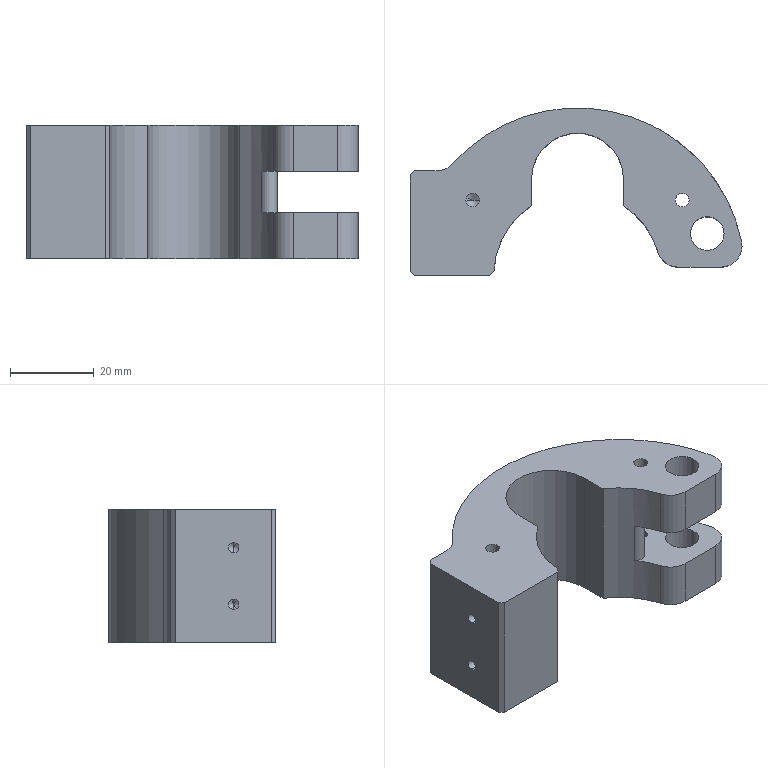Part | STEP file | Support intermediate piece-upper | 1 solid | 49 faces | box 79.293 x 40 x 32 mm | volume 45814 mm3 | cylinder 26 | plane 15 | cone 8 | commonest cylinder face diameters 3.3 x8 10 x5 2.5 x4 8 x4 40 x2 4 x1